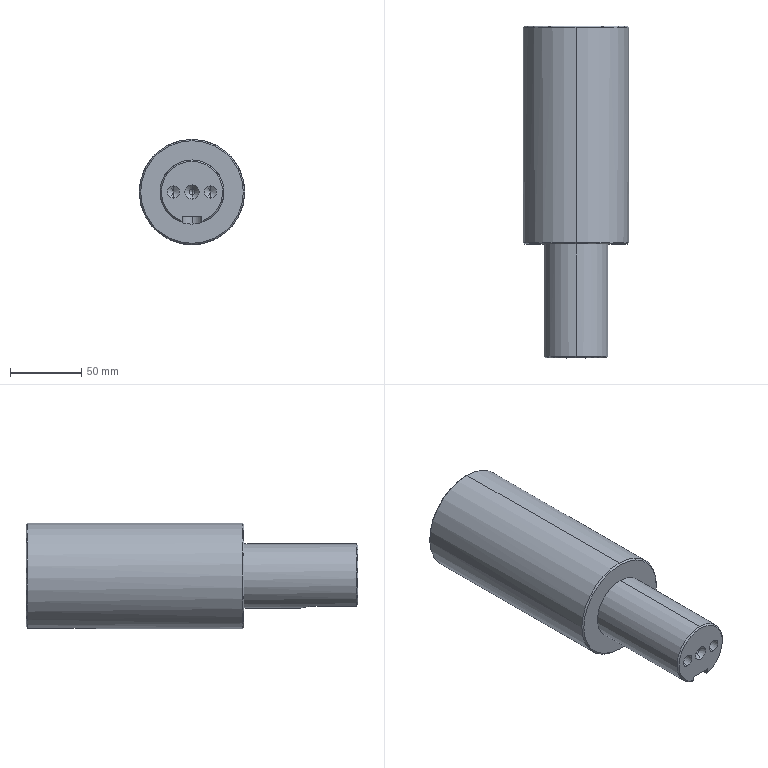Part | SolidWorks | features ICE 3, 3DProfileFeature 2, Chamfer 2, Fillet 2, HoleWzd 2, Extrusion 1 | 1 solid | 36 faces | box 74 x 233 x 74 mm | volume 776364 mm3 | cylinder 14 | cone 13 | plane 9 | commonest cylinder face diameters 8.5 x4 4 x2 10 x2 14 x2 45 x2 74 x2
STEP:
#1=CARTESIAN_POINT('',(0.,3.451,2.));
#2=VERTEX_POINT('',#1);
#3=CARTESIAN_POINT('',(0.,3.451,-2.));
#4=VERTEX_POINT('',#3);
#5=CARTESIAN_POINT('',(0.,3.451,0.));
#6=DIRECTION('',(0.,-1.,0.));
#7=DIRECTION('',(0.,0.,-1.));
#8=AXIS2_PLACEMENT_3D('',#5,#6,#7);
#9=CIRCLE('',#8,2.);
#10=EDGE_CURVE('',#2,#4,#9,.T.);
#11=ORIENTED_EDGE('',*,*,#10,.F.);
#12=CARTESIAN_POINT('',(0.,0.,5.));
#13=VERTEX_POINT('',#12);
#14=CARTESIAN_POINT('',(0.,0.,5.));
#15=DIRECTION('',(0.,-0.7547,0.6561));
#16=VECTOR('',#15,1000.);
#17=LINE('',#14,#16);
#18=EDGE_CURVE('',#2,#13,#17,.T.);
#19=ORIENTED_EDGE('',*,*,#18,.T.);
#20=CARTESIAN_POINT('',(0.,0.,-5.));
#21=VERTEX_POINT('',#20);
#22=CARTESIAN_POINT('',(0.,0.,0.));
#23=DIRECTION('',(0.,-1.,0.));
#24=DIRECTION('',(0.,0.,-1.));
#25=AXIS2_PLACEMENT_3D('',#22,#23,#24);
#26=CIRCLE('',#25,5.);
#27=EDGE_CURVE('',#13,#21,#26,.T.);
#28=ORIENTED_EDGE('',*,*,#27,.T.);
#29=CARTESIAN_POINT('',(0.,0.,-5.));
#30=DIRECTION('',(0.,-0.7547,-0.6561));
#31=VECTOR('',#30,1000.);
#32=LINE('',#29,#31);
#33=EDGE_CURVE('',#4,#21,#32,.T.);
#34=ORIENTED_EDGE('',*,*,#33,.F.);
#35=EDGE_LOOP('',(#11,#19,#28,#34));
#36=FACE_OUTER_BOUND('',#35,.T.);
#37=CARTESIAN_POINT('',(0.,0.,0.));
#38=DIRECTION('',(0.,-1.,0.));
#39=DIRECTION('',(0.,0.,-1.));
#40=AXIS2_PLACEMENT_3D('',#37,#38,#39);
#41=CONICAL_SURFACE('',#40,5.,0.7156);
#42=ADVANCED_FACE('',(#36),#41,.F.);
#43=CARTESIAN_POINT('',(0.,10.,2.));
#44=VERTEX_POINT('',#43);
#45=CARTESIAN_POINT('',(0.,10.,-2.));
#46=VERTEX_POINT('',#45);
#47=CARTESIAN_POINT('',(0.,10.,0.));
#48=DIRECTION('',(0.,-1.,0.));
#49=DIRECTION('',(0.,0.,-1.));
#50=AXIS2_PLACEMENT_3D('',#47,#48,#49);
#51=CIRCLE('',#50,2.);
#52=EDGE_CURVE('',#44,#46,#51,.T.);
#53=ORIENTED_EDGE('',*,*,#52,.F.);
#54=CARTESIAN_POINT('',(0.,0.,2.));
#55=DIRECTION('',(0.,-1.,0.));
#56=VECTOR('',#55,1000.);
#57=LINE('',#54,#56);
#58=EDGE_CURVE('',#44,#2,#57,.T.);
#59=ORIENTED_EDGE('',*,*,#58,.T.);
#60=ORIENTED_EDGE('',*,*,#10,.T.);
#61=CARTESIAN_POINT('',(0.,0.,-2.));
#62=DIRECTION('',(0.,-1.,0.));
#63=VECTOR('',#62,1000.);
#64=LINE('',#61,#63);
#65=EDGE_CURVE('',#46,#4,#64,.T.);
#66=ORIENTED_EDGE('',*,*,#65,.F.);
#67=EDGE_LOOP('',(#53,#59,#60,#66));
#68=FACE_OUTER_BOUND('',#67,.T.);
#69=CARTESIAN_POINT('',(0.,0.,0.));
#70=DIRECTION('',(0.,-1.,0.));
#71=DIRECTION('',(0.,0.,-1.));
#72=AXIS2_PLACEMENT_3D('',#69,#70,#71);
#73=CYLINDRICAL_SURFACE('',#72,2.);
#74=ADVANCED_FACE('',(#68),#73,.F.);
#75=CARTESIAN_POINT('',(0.,11.202,0.));
#76=VERTEX_POINT('',#75);
#77=CARTESIAN_POINT('',(0.,10.,-2.));
#78=DIRECTION('',(0.,-0.515,-0.8572));
#79=VECTOR('',#78,1000.);
#80=LINE('',#77,#79);
#81=EDGE_CURVE('',#76,#46,#80,.T.);
#82=ORIENTED_EDGE('',*,*,#81,.F.);
#83=CARTESIAN_POINT('',(0.,10.,2.));
#84=DIRECTION('',(0.,-0.515,0.8572));
#85=VECTOR('',#84,1000.);
#86=LINE('',#83,#85);
#87=EDGE_CURVE('',#76,#44,#86,.T.);
#88=ORIENTED_EDGE('',*,*,#87,.T.);
#89=ORIENTED_EDGE('',*,*,#52,.T.);
#90=EDGE_LOOP('',(#82,#88,#89));
#91=FACE_OUTER_BOUND('',#90,.T.);
#92=CARTESIAN_POINT('',(0.,10.,0.));
#93=DIRECTION('',(0.,-1.,0.));
#94=DIRECTION('',(0.,0.,-1.));
#95=AXIS2_PLACEMENT_3D('',#92,#93,#94);
#96=CONICAL_SURFACE('',#95,2.,1.03);
#97=ADVANCED_FACE('',(#91),#96,.F.);
#98=CARTESIAN_POINT('',(0.,80.,-36.));
#99=VERTEX_POINT('',#98);
#100=CARTESIAN_POINT('',(0.,80.,36.));
#101=VERTEX_POINT('',#100);
#102=CARTESIAN_POINT('',(0.,80.,0.));
#103=DIRECTION('',(0.,-1.,0.));
#104=DIRECTION('',(0.,0.,1.));
#105=AXIS2_PLACEMENT_3D('',#102,#103,#104);
#106=CIRCLE('',#105,36.);
#107=EDGE_CURVE('',#99,#101,#106,.T.);
#108=ORIENTED_EDGE('',*,*,#107,.F.);
#109=CARTESIAN_POINT('',(0.,81.,-37.));
#110=VERTEX_POINT('',#109);
#111=CARTESIAN_POINT('',(0.,81.,-37.));
#112=DIRECTION('',(0.,0.7071,-0.7071));
#113=VECTOR('',#112,1000.);
#114=LINE('',#111,#113);
#115=EDGE_CURVE('',#99,#110,#114,.T.);
#116=ORIENTED_EDGE('',*,*,#115,.T.);
#117=CARTESIAN_POINT('',(0.,81.,37.));
#118=VERTEX_POINT('',#117);
#119=CARTESIAN_POINT('',(0.,81.,0.));
#120=DIRECTION('',(0.,1.,0.));
#121=DIRECTION('',(0.,0.,1.));
#122=AXIS2_PLACEMENT_3D('',#119,#120,#121);
#123=CIRCLE('',#122,37.);
#124=EDGE_CURVE('',#118,#110,#123,.T.);
#125=ORIENTED_EDGE('',*,*,#124,.F.);
#126=CARTESIAN_POINT('',(0.,81.,37.));
#127=DIRECTION('',(0.,0.7071,0.7071));
#128=VECTOR('',#127,1000.);
#129=LINE('',#126,#128);
#130=EDGE_CURVE('',#101,#118,#129,.T.);
#131=ORIENTED_EDGE('',*,*,#130,.F.);
#132=EDGE_LOOP('',(#108,#116,#125,#131));
#133=FACE_OUTER_BOUND('',#132,.T.);
#134=CARTESIAN_POINT('',(0.,81.,0.));
#135=DIRECTION('',(0.,1.,0.));
#136=DIRECTION('',(0.,0.,1.));
#137=AXIS2_PLACEMENT_3D('',#134,#135,#136);
#138=CONICAL_SURFACE('',#137,37.,0.7854);
#139=ADVANCED_FACE('',(#133),#138,.T.);
#140=CARTESIAN_POINT('',(5.,232.,-36.661));
#141=VERTEX_POINT('',#140);
#142=CARTESIAN_POINT('',(0.,232.,37.));
#143=VERTEX_POINT('',#142);
#144=CARTESIAN_POINT('',(0.,232.,0.));
#145=DIRECTION('',(0.,-1.,0.));
#146=DIRECTION('',(0.,0.,1.));
#147=AXIS2_PLACEMENT_3D('',#144,#145,#146);
#148=CIRCLE('',#147,37.);
#149=EDGE_CURVE('',#141,#143,#148,.T.);
#150=ORIENTED_EDGE('',*,*,#149,.T.);
#151=CARTESIAN_POINT('',(0.,233.,37.));
#152=DIRECTION('',(0.,-1.,0.));
#153=VECTOR('',#152,1000.);
#154=LINE('',#151,#153);
#155=EDGE_CURVE('',#143,#118,#154,.T.);
#156=ORIENTED_EDGE('',*,*,#155,.T.);
#157=ORIENTED_EDGE('',*,*,#124,.T.);
#158=CARTESIAN_POINT('',(0.,183.,-37.));
#159=VERTEX_POINT('',#158);
#160=CARTESIAN_POINT('',(0.,233.,-37.));
#161=DIRECTION('',(0.,-1.,0.));
#162=VECTOR('',#161,1000.);
#163=LINE('',#160,#162);
#164=EDGE_CURVE('',#159,#110,#163,.T.);
#165=ORIENTED_EDGE('',*,*,#164,.F.);
#166=CARTESIAN_POINT('',(5.,188.,-36.661));
#167=VERTEX_POINT('',#166);
#168=CARTESIAN_POINT('',(0.,183.,-37.));
#169=CARTESIAN_POINT('',(0.3305,183.,-37.));
#170=CARTESIAN_POINT('',(0.6555,183.032,-36.996));
#171=CARTESIAN_POINT('',(1.135,183.128,-36.983));
#172=CARTESIAN_POINT('',(1.293,183.167,-36.978));
#173=CARTESIAN_POINT('',(1.607,183.263,-36.965));
#174=CARTESIAN_POINT('',(1.764,183.318,-36.958));
#175=CARTESIAN_POINT('',(2.217,183.507,-36.935));
#176=CARTESIAN_POINT('',(2.504,183.66,-36.916));
#177=CARTESIAN_POINT('',(3.047,184.022,-36.875));
#178=CARTESIAN_POINT('',(3.304,184.233,-36.853));
#179=CARTESIAN_POINT('',(3.765,184.693,-36.809));
#180=CARTESIAN_POINT('',(3.972,184.945,-36.787));
#181=CARTESIAN_POINT('',(4.337,185.491,-36.745));
#182=CARTESIAN_POINT('',(4.492,185.781,-36.726));
#183=CARTESIAN_POINT('',(4.742,186.382,-36.695));
#184=CARTESIAN_POINT('',(4.838,186.696,-36.682));
#185=CARTESIAN_POINT('',(4.968,187.343,-36.665));
#186=CARTESIAN_POINT('',(5.,187.669,-36.661));
#187=CARTESIAN_POINT('',(5.,188.,-36.661));
#188=B_SPLINE_CURVE_WITH_KNOTS('',3,(#168,#169,#170,#171,#172,#173,#174,#175,#176,#177,#178,#179,#180,#181,#182,#183,#184,#185,#186,#187),.UNSPECIFIED.,.F.,.F.,(4,2,2,2,2,2,2,2,2,4),(0.,0.0009775,0.001466,0.001955,0.002932,0.00391,0.004887,0.005865,0.006842,0.00782),.UNSPECIFIED.);
#189=EDGE_CURVE('',#159,#167,#188,.T.);
#190=ORIENTED_EDGE('',*,*,#189,.T.);
#191=CARTESIAN_POINT('',(5.,233.,-36.661));
#192=DIRECTION('',(0.,1.,0.));
#193=VECTOR('',#192,1000.);
#194=LINE('',#191,#193);
#195=EDGE_CURVE('',#167,#141,#194,.T.);
#196=ORIENTED_EDGE('',*,*,#195,.T.);
#197=EDGE_LOOP('',(#150,#156,#157,#165,#190,#196));
#198=FACE_OUTER_BOUND('',#197,.T.);
#199=CARTESIAN_POINT('',(0.,233.,0.));
#200=DIRECTION('',(0.,-1.,0.));
#201=DIRECTION('',(0.,0.,-1.));
#202=AXIS2_PLACEMENT_3D('',#199,#200,#201);
#203=CYLINDRICAL_SURFACE('',#202,37.);
#204=ADVANCED_FACE('',(#198),#203,.T.);
#205=CARTESIAN_POINT('',(0.,0.,21.5));
#206=VERTEX_POINT('',#205);
#207=CARTESIAN_POINT('',(-7.,0.,-20.329));
#208=VERTEX_POINT('',#207);
#209=CARTESIAN_POINT('',(0.,0.,0.));
#210=DIRECTION('',(0.,-1.,0.));
#211=DIRECTION('',(0.,0.,1.));
#212=AXIS2_PLACEMENT_3D('',#209,#210,#211);
#213=CIRCLE('',#212,21.5);
#214=EDGE_CURVE('',#206,#208,#213,.T.);
#215=ORIENTED_EDGE('',*,*,#214,.F.);
#216=CARTESIAN_POINT('',(0.,1.,22.5));
#217=VERTEX_POINT('',#216);
#218=CARTESIAN_POINT('',(0.,1.,22.5));
#219=DIRECTION('',(0.,0.7071,0.7071));
#220=VECTOR('',#219,1000.);
#221=LINE('',#218,#220);
#222=EDGE_CURVE('',#206,#217,#221,.T.);
#223=ORIENTED_EDGE('',*,*,#222,.T.);
#224=CARTESIAN_POINT('',(-7.,1.,-21.383));
#225=VERTEX_POINT('',#224);
#226=CARTESIAN_POINT('',(0.,1.,0.));
#227=DIRECTION('',(0.,1.,0.));
#228=DIRECTION('',(0.,0.,1.));
#229=AXIS2_PLACEMENT_3D('',#226,#227,#228);
#230=CIRCLE('',#229,22.5);
#231=EDGE_CURVE('',#225,#217,#230,.T.);
#232=ORIENTED_EDGE('',*,*,#231,.F.);
#233=CARTESIAN_POINT('',(-7.,0.,-20.329));
#234=CARTESIAN_POINT('',(-7.,0.3329,-20.681));
#235=CARTESIAN_POINT('',(-7.,0.6662,-21.032));
#236=CARTESIAN_POINT('',(-7.,1.,-21.383));
#237=B_SPLINE_CURVE_WITH_KNOTS('',3,(#233,#234,#235,#236),.UNSPECIFIED.,.F.,.F.,(4,4),(0.,0.001454),.UNSPECIFIED.);
#238=EDGE_CURVE('',#208,#225,#237,.T.);
#239=ORIENTED_EDGE('',*,*,#238,.F.);
#240=EDGE_LOOP('',(#215,#223,#232,#239));
#241=FACE_OUTER_BOUND('',#240,.T.);
#242=CARTESIAN_POINT('',(0.,1.,0.));
#243=DIRECTION('',(0.,1.,0.));
#244=DIRECTION('',(0.,0.,1.));
#245=AXIS2_PLACEMENT_3D('',#242,#243,#244);
#246=CONICAL_SURFACE('',#245,22.5,0.7854);
#247=ADVANCED_FACE('',(#241),#246,.T.);
#248=CARTESIAN_POINT('',(-13.,27.5,4.25));
#249=VERTEX_POINT('',#248);
#250=CARTESIAN_POINT('',(-13.,27.5,-4.25));
#251=VERTEX_POINT('',#250);
#252=CARTESIAN_POINT('',(-13.,27.5,0.));
#253=DIRECTION('',(0.,-1.,0.));
#254=DIRECTION('',(0.,0.,-1.));
#255=AXIS2_PLACEMENT_3D('',#252,#253,#254);
#256=CIRCLE('',#255,4.25);
#257=EDGE_CURVE('',#249,#251,#256,.T.);
#258=ORIENTED_EDGE('',*,*,#257,.F.);
#259=CARTESIAN_POINT('',(-13.,0.,4.25));
#260=VERTEX_POINT('',#259);
#261=CARTESIAN_POINT('',(-13.,0.,4.25));
#262=DIRECTION('',(0.,-1.,0.));
#263=VECTOR('',#262,1000.);
#264=LINE('',#261,#263);
#265=EDGE_CURVE('',#249,#260,#264,.T.);
#266=ORIENTED_EDGE('',*,*,#265,.T.);
#267=CARTESIAN_POINT('',(-13.,0.,-4.25));
#268=VERTEX_POINT('',#267);
#269=CARTESIAN_POINT('',(-13.,0.,0.));
#270=DIRECTION('',(0.,-1.,0.));
#271=DIRECTION('',(0.,0.,-1.));
#272=AXIS2_PLACEMENT_3D('',#269,#270,#271);
#273=CIRCLE('',#272,4.25);
#274=EDGE_CURVE('',#260,#268,#273,.T.);
#275=ORIENTED_EDGE('',*,*,#274,.T.);
#276=CARTESIAN_POINT('',(-13.,0.,-4.25));
#277=DIRECTION('',(0.,-1.,0.));
#278=VECTOR('',#277,1000.);
#279=LINE('',#276,#278);
#280=EDGE_CURVE('',#251,#268,#279,.T.);
#281=ORIENTED_EDGE('',*,*,#280,.F.);
#282=EDGE_LOOP('',(#258,#266,#275,#281));
#283=FACE_OUTER_BOUND('',#282,.T.);
#284=CARTESIAN_POINT('',(-13.,0.,0.));
#285=DIRECTION('',(0.,-1.,0.));
#286=DIRECTION('',(0.,0.,-1.));
#287=AXIS2_PLACEMENT_3D('',#284,#285,#286);
#288=CYLINDRICAL_SURFACE('',#287,4.25);
#289=ADVANCED_FACE('',(#283),#288,.F.);
#290=CARTESIAN_POINT('',(-13.,30.054,0.));
#291=VERTEX_POINT('',#290);
#292=CARTESIAN_POINT('',(-13.,27.5,-4.25));
#293=DIRECTION('',(0.,-0.515,-0.8572));
#294=VECTOR('',#293,1000.);
#295=LINE('',#292,#294);
#296=EDGE_CURVE('',#291,#251,#295,.T.);
#297=ORIENTED_EDGE('',*,*,#296,.F.);
#298=CARTESIAN_POINT('',(-13.,27.5,4.25));
#299=DIRECTION('',(0.,-0.515,0.8572));
#300=VECTOR('',#299,1000.);
#301=LINE('',#298,#300);
#302=EDGE_CURVE('',#291,#249,#301,.T.);
#303=ORIENTED_EDGE('',*,*,#302,.T.);
#304=ORIENTED_EDGE('',*,*,#257,.T.);
#305=EDGE_LOOP('',(#297,#303,#304));
#306=FACE_OUTER_BOUND('',#305,.T.);
#307=CARTESIAN_POINT('',(-13.,27.5,0.));
#308=DIRECTION('',(0.,-1.,0.));
#309=DIRECTION('',(0.,0.,-1.));
#310=AXIS2_PLACEMENT_3D('',#307,#308,#309);
#311=CONICAL_SURFACE('',#310,4.25,1.03);
#312=ADVANCED_FACE('',(#306),#311,.F.);
#313=CARTESIAN_POINT('',(13.,27.5,4.25));
#314=VERTEX_POINT('',#313);
#315=CARTESIAN_POINT('',(13.,27.5,-4.25));
#316=VERTEX_POINT('',#315);
#317=CARTESIAN_POINT('',(13.,27.5,0.));
#318=DIRECTION('',(0.,-1.,0.));
#319=DIRECTION('',(0.,0.,-1.));
#320=AXIS2_PLACEMENT_3D('',#317,#318,#319);
#321=CIRCLE('',#320,4.25);
#322=EDGE_CURVE('',#314,#316,#321,.T.);
#323=ORIENTED_EDGE('',*,*,#322,.F.);
#324=CARTESIAN_POINT('',(13.,0.,4.25));
#325=VERTEX_POINT('',#324);
#326=CARTESIAN_POINT('',(13.,0.,4.25));
#327=DIRECTION('',(0.,-1.,0.));
#328=VECTOR('',#327,1000.);
#329=LINE('',#326,#328);
#330=EDGE_CURVE('',#314,#325,#329,.T.);
#331=ORIENTED_EDGE('',*,*,#330,.T.);
#332=CARTESIAN_POINT('',(13.,0.,-4.25));
#333=VERTEX_POINT('',#332);
#334=CARTESIAN_POINT('',(13.,0.,0.));
#335=DIRECTION('',(0.,-1.,0.));
#336=DIRECTION('',(0.,0.,-1.));
#337=AXIS2_PLACEMENT_3D('',#334,#335,#336);
#338=CIRCLE('',#337,4.25);
#339=EDGE_CURVE('',#325,#333,#338,.T.);
#340=ORIENTED_EDGE('',*,*,#339,.T.);
#341=CARTESIAN_POINT('',(13.,0.,-4.25));
#342=DIRECTION('',(0.,-1.,0.));
#343=VECTOR('',#342,1000.);
#344=LINE('',#341,#343);
#345=EDGE_CURVE('',#316,#333,#344,.T.);
#346=ORIENTED_EDGE('',*,*,#345,.F.);
#347=EDGE_LOOP('',(#323,#331,#340,#346));
#348=FACE_OUTER_BOUND('',#347,.T.);
#349=CARTESIAN_POINT('',(13.,0.,0.));
#350=DIRECTION('',(0.,-1.,0.));
#351=DIRECTION('',(0.,0.,-1.));
#352=AXIS2_PLACEMENT_3D('',#349,#350,#351);
#353=CYLINDRICAL_SURFACE('',#352,4.25);
#354=ADVANCED_FACE('',(#348),#353,.F.);
#355=CARTESIAN_POINT('',(13.,30.054,0.));
#356=VERTEX_POINT('',#355);
#357=CARTESIAN_POINT('',(13.,27.5,-4.25));
#358=DIRECTION('',(0.,-0.515,-0.8572));
#359=VECTOR('',#358,1000.);
#360=LINE('',#357,#359);
#361=EDGE_CURVE('',#356,#316,#360,.T.);
#362=ORIENTED_EDGE('',*,*,#361,.F.);
#363=CARTESIAN_POINT('',(13.,27.5,4.25));
#364=DIRECTION('',(0.,-0.515,0.8572));
#365=VECTOR('',#364,1000.);
#366=LINE('',#363,#365);
#367=EDGE_CURVE('',#356,#314,#366,.T.);
#368=ORIENTED_EDGE('',*,*,#367,.T.);
#369=ORIENTED_EDGE('',*,*,#322,.T.);
#370=EDGE_LOOP('',(#362,#368,#369));
#371=FACE_OUTER_BOUND('',#370,.T.);
#372=CARTESIAN_POINT('',(13.,27.5,0.));
#373=DIRECTION('',(0.,-1.,0.));
#374=DIRECTION('',(0.,0.,-1.));
#375=AXIS2_PLACEMENT_3D('',#372,#373,#374);
#376=CONICAL_SURFACE('',#375,4.25,1.03);
#377=ADVANCED_FACE('',(#371),#376,.F.);
#378=CARTESIAN_POINT('',(0.,80.,22.5));
#379=VERTEX_POINT('',#378);
#380=CARTESIAN_POINT('',(0.,80.,-22.5));
#381=VERTEX_POINT('',#380);
#382=CARTESIAN_POINT('',(0.,80.,0.));
#383=DIRECTION('',(0.,1.,0.));
#384=DIRECTION('',(0.,0.,1.));
#385=AXIS2_PLACEMENT_3D('',#382,#383,#384);
#386=CIRCLE('',#385,22.5);
#387=EDGE_CURVE('',#379,#381,#386,.T.);
#388=ORIENTED_EDGE('',*,*,#387,.F.);
#389=CARTESIAN_POINT('',(0.,40.,22.5));
#390=DIRECTION('',(0.,-1.,0.));
#391=VECTOR('',#390,1000.);
#392=LINE('',#389,#391);
#393=EDGE_CURVE('',#379,#217,#392,.T.);
#394=ORIENTED_EDGE('',*,*,#393,.T.);
#395=CARTESIAN_POINT('',(7.,1.,-21.383));
#396=VERTEX_POINT('',#395);
#397=CARTESIAN_POINT('',(0.,1.,0.));
#398=DIRECTION('',(0.,1.,0.));
#399=DIRECTION('',(0.,0.,1.));
#400=AXIS2_PLACEMENT_3D('',#397,#398,#399);
#401=CIRCLE('',#400,22.5);
#402=EDGE_CURVE('',#217,#396,#401,.T.);
#403=ORIENTED_EDGE('',*,*,#402,.T.);
#404=CARTESIAN_POINT('',(7.,33.,-21.383));
#405=VERTEX_POINT('',#404);
#406=CARTESIAN_POINT('',(7.,40.,-21.383));
#407=DIRECTION('',(0.,-1.,0.));
#408=VECTOR('',#407,1000.);
#409=LINE('',#406,#408);
#410=EDGE_CURVE('',#405,#396,#409,.T.);
#411=ORIENTED_EDGE('',*,*,#410,.F.);
#412=CARTESIAN_POINT('',(0.,40.,-22.5));
#413=VERTEX_POINT('',#412);
#414=CARTESIAN_POINT('',(7.,33.,-21.383));
#415=CARTESIAN_POINT('',(7.,33.465,-21.383));
#416=CARTESIAN_POINT('',(6.954,33.922,-21.399));
#417=CARTESIAN_POINT('',(6.82,34.596,-21.442));
#418=CARTESIAN_POINT('',(6.764,34.818,-21.459));
#419=CARTESIAN_POINT('',(6.629,35.259,-21.501));
#420=CARTESIAN_POINT('',(6.551,35.478,-21.525));
#421=CARTESIAN_POINT('',(6.287,36.112,-21.605));
#422=CARTESIAN_POINT('',(6.072,36.513,-21.667));
#423=CARTESIAN_POINT('',(5.692,37.081,-21.769));
#424=CARTESIAN_POINT('',(5.554,37.266,-21.804));
#425=CARTESIAN_POINT('',(5.264,37.62,-21.876));
#426=CARTESIAN_POINT('',(5.112,37.788,-21.912));
#427=CARTESIAN_POINT('',(4.631,38.269,-22.021));
#428=CARTESIAN_POINT('',(4.281,38.558,-22.092));
#429=CARTESIAN_POINT('',(3.517,39.07,-22.227));
#430=CARTESIAN_POINT('',(3.115,39.285,-22.287));
#431=CARTESIAN_POINT('',(2.484,39.548,-22.363));
#432=CARTESIAN_POINT('',(2.269,39.626,-22.386));
#433=CARTESIAN_POINT('',(1.83,39.76,-22.427));
#434=CARTESIAN_POINT('',(1.604,39.818,-22.444));
#435=CARTESIAN_POINT('',(0.9245,39.954,-22.486));
#436=CARTESIAN_POINT('',(0.4653,40.,-22.5));
#437=CARTESIAN_POINT('',(0.,40.,-22.5));
#438=B_SPLINE_CURVE_WITH_KNOTS('',3,(#414,#415,#416,#417,#418,#419,#420,#421,#422,#423,#424,#425,#426,#427,#428,#429,#430,#431,#432,#433,#434,#435,#436,#437),.UNSPECIFIED.,.F.,.F.,(4,2,2,2,2,2,2,2,2,2,2,4),(0.,0.001375,0.002063,0.002751,0.004126,0.004814,0.005502,0.006877,0.008253,0.008941,0.009628,0.011),.UNSPECIFIED.);
#439=EDGE_CURVE('',#405,#413,#438,.T.);
#440=ORIENTED_EDGE('',*,*,#439,.T.);
#441=CARTESIAN_POINT('',(0.,40.,-22.5));
#442=DIRECTION('',(0.,-1.,0.));
#443=VECTOR('',#442,1000.);
#444=LINE('',#441,#443);
#445=EDGE_CURVE('',#381,#413,#444,.T.);
#446=ORIENTED_EDGE('',*,*,#445,.F.);
#447=EDGE_LOOP('',(#388,#394,#403,#411,#440,#446));
#448=FACE_OUTER_BOUND('',#447,.T.);
#449=CARTESIAN_POINT('',(0.,40.,0.));
#450=DIRECTION('',(0.,-1.,0.));
#451=DIRECTION('',(0.,0.,-1.));
#452=AXIS2_PLACEMENT_3D('',#449,#450,#451);
#453=CYLINDRICAL_SURFACE('',#452,22.5);
#454=ADVANCED_FACE('',(#448),#453,.T.);
#455=ORIENTED_EDGE('',*,*,#393,.F.);
#456=CARTESIAN_POINT('',(0.,80.,0.));
#457=DIRECTION('',(0.,1.,0.));
#458=DIRECTION('',(0.,0.,1.));
#459=AXIS2_PLACEMENT_3D('',#456,#457,#458);
#460=CIRCLE('',#459,22.5);
#461=EDGE_CURVE('',#381,#379,#460,.T.);
#462=ORIENTED_EDGE('',*,*,#461,.F.);
#463=ORIENTED_EDGE('',*,*,#445,.T.);
#464=CARTESIAN_POINT('',(-7.,33.,-21.383));
#465=VERTEX_POINT('',#464);
#466=CARTESIAN_POINT('',(0.,40.,-22.5));
#467=CARTESIAN_POINT('',(-0.4653,40.,-22.5));
#468=CARTESIAN_POINT('',(-0.9223,39.954,-22.486));
#469=CARTESIAN_POINT('',(-1.596,39.819,-22.444));
#470=CARTESIAN_POINT('',(-1.818,39.764,-22.427));
#471=CARTESIAN_POINT('',(-2.26,39.629,-22.387));
#472=CARTESIAN_POINT('',(-2.478,39.551,-22.364));
#473=CARTESIAN_POINT('',(-3.113,39.287,-22.288));
#474=CARTESIAN_POINT('',(-3.513,39.072,-22.227));
#475=CARTESIAN_POINT('',(-4.082,38.691,-22.127));
#476=CARTESIAN_POINT('',(-4.267,38.554,-22.092));
#477=CARTESIAN_POINT('',(-4.621,38.263,-22.021));
#478=CARTESIAN_POINT('',(-4.789,38.111,-21.985));
#479=CARTESIAN_POINT('',(-5.27,37.63,-21.877));
#480=CARTESIAN_POINT('',(-5.558,37.28,-21.804));
#481=CARTESIAN_POINT('',(-6.07,36.516,-21.667));
#482=CARTESIAN_POINT('',(-6.286,36.114,-21.605));
#483=CARTESIAN_POINT('',(-6.548,35.484,-21.526));
#484=CARTESIAN_POINT('',(-6.626,35.269,-21.502));
#485=CARTESIAN_POINT('',(-6.76,34.83,-21.46));
#486=CARTESIAN_POINT('',(-6.818,34.604,-21.442));
#487=CARTESIAN_POINT('',(-6.954,33.924,-21.399));
#488=CARTESIAN_POINT('',(-7.,33.465,-21.383));
#489=CARTESIAN_POINT('',(-7.,33.,-21.383));
#490=B_SPLINE_CURVE_WITH_KNOTS('',3,(#466,#467,#468,#469,#470,#471,#472,#473,#474,#475,#476,#477,#478,#479,#480,#481,#482,#483,#484,#485,#486,#487,#488,#489),.UNSPECIFIED.,.F.,.F.,(4,2,2,2,2,2,2,2,2,2,2,4),(0.,0.001376,0.002063,0.002751,0.004127,0.004814,0.005502,0.006878,0.008253,0.008941,0.009629,0.011),.UNSPECIFIED.);
#491=EDGE_CURVE('',#413,#465,#490,.T.);
#492=ORIENTED_EDGE('',*,*,#491,.T.);
#493=CARTESIAN_POINT('',(-7.,40.,-21.383));
#494=DIRECTION('',(0.,-1.,0.));
#495=VECTOR('',#494,1000.);
#496=LINE('',#493,#495);
#497=EDGE_CURVE('',#465,#225,#496,.T.);
#498=ORIENTED_EDGE('',*,*,#497,.T.);
#499=ORIENTED_EDGE('',*,*,#231,.T.);
#500=EDGE_LOOP('',(#455,#462,#463,#492,#498,#499));
#501=FACE_OUTER_BOUND('',#500,.T.);
#502=CARTESIAN_POINT('',(0.,40.,0.));
#503=DIRECTION('',(0.,-1.,0.));
#504=DIRECTION('',(0.,0.,-1.));
#505=AXIS2_PLACEMENT_3D('',#502,#503,#504);
#506=CYLINDRICAL_SURFACE('',#505,22.5);
#507=ADVANCED_FACE('',(#501),#506,.T.);
#508=ORIENTED_EDGE('',*,*,#410,.T.);
#509=CARTESIAN_POINT('',(7.,0.,-20.329));
#510=VERTEX_POINT('',#509);
#511=CARTESIAN_POINT('',(7.,1.,-21.383));
#512=CARTESIAN_POINT('',(7.,0.6662,-21.032));
#513=CARTESIAN_POINT('',(7.,0.3329,-20.681));
#514=CARTESIAN_POINT('',(7.,0.,-20.329));
#515=B_SPLINE_CURVE_WITH_KNOTS('',3,(#511,#512,#513,#514),.UNSPECIFIED.,.F.,.F.,(4,4),(0.,0.001454),.UNSPECIFIED.);
#516=EDGE_CURVE('',#396,#510,#515,.T.);
#517=ORIENTED_EDGE('',*,*,#516,.T.);
#518=CARTESIAN_POINT('',(7.,0.,-17.));
#519=VERTEX_POINT('',#518);
#520=CARTESIAN_POINT('',(7.,0.,-21.383));
#521=DIRECTION('',(0.,0.,1.));
#522=VECTOR('',#521,1000.);
#523=LINE('',#520,#522);
#524=EDGE_CURVE('',#510,#519,#523,.T.);
#525=ORIENTED_EDGE('',*,*,#524,.T.);
#526=CARTESIAN_POINT('',(7.,33.,-17.));
#527=VERTEX_POINT('',#526);
#528=CARTESIAN_POINT('',(7.,40.,-17.));
#529=DIRECTION('',(0.,-1.,0.));
#530=VECTOR('',#529,1000.);
#531=LINE('',#528,#530);
#532=EDGE_CURVE('',#527,#519,#531,.T.);
#533=ORIENTED_EDGE('',*,*,#532,.F.);
#534=CARTESIAN_POINT('',(7.,33.,-21.383));
#535=DIRECTION('',(0.,0.,-1.));
#536=VECTOR('',#535,1000.);
#537=LINE('',#534,#536);
#538=EDGE_CURVE('',#527,#405,#537,.T.);
#539=ORIENTED_EDGE('',*,*,#538,.T.);
#540=EDGE_LOOP('',(#508,#517,#525,#533,#539));
#541=FACE_OUTER_BOUND('',#540,.T.);
#542=CARTESIAN_POINT('',(7.,40.,-21.383));
#543=DIRECTION('',(1.,0.,0.));
#544=DIRECTION('',(0.,0.,-1.));
#545=AXIS2_PLACEMENT_3D('',#542,#543,#544);
#546=PLANE('',#545);
#547=ADVANCED_FACE('',(#541),#546,.F.);
#548=CARTESIAN_POINT('',(-7.,33.,-17.));
#549=VERTEX_POINT('',#548);
#550=CARTESIAN_POINT('',(-7.,0.,-17.));
#551=VERTEX_POINT('',#550);
#552=CARTESIAN_POINT('',(-7.,40.,-17.));
#553=DIRECTION('',(0.,-1.,0.));
#554=VECTOR('',#553,1000.);
#555=LINE('',#552,#554);
#556=EDGE_CURVE('',#549,#551,#555,.T.);
#557=ORIENTED_EDGE('',*,*,#556,.F.);
#558=CARTESIAN_POINT('',(0.,40.,-17.));
#559=VERTEX_POINT('',#558);
#560=CARTESIAN_POINT('',(0.,33.,-17.));
#561=DIRECTION('',(0.,0.,-1.));
#562=DIRECTION('',(1.,0.,0.));
#563=AXIS2_PLACEMENT_3D('',#560,#561,#562);
#564=CIRCLE('',#563,7.);
#565=EDGE_CURVE('',#549,#559,#564,.T.);
#566=ORIENTED_EDGE('',*,*,#565,.T.);
#567=CARTESIAN_POINT('',(0.,33.,-17.));
#568=DIRECTION('',(0.,0.,-1.));
#569=DIRECTION('',(1.,0.,0.));
#570=AXIS2_PLACEMENT_3D('',#567,#568,#569);
#571=CIRCLE('',#570,7.);
#572=EDGE_CURVE('',#559,#527,#571,.T.);
#573=ORIENTED_EDGE('',*,*,#572,.T.);
#574=ORIENTED_EDGE('',*,*,#532,.T.);
#575=CARTESIAN_POINT('',(-7.,0.,-17.));
#576=DIRECTION('',(-1.,0.,0.));
#577=VECTOR('',#576,1000.);
#578=LINE('',#575,#577);
#579=EDGE_CURVE('',#519,#551,#578,.T.);
#580=ORIENTED_EDGE('',*,*,#579,.T.);
#581=EDGE_LOOP('',(#557,#566,#573,#574,#580));
#582=FACE_OUTER_BOUND('',#581,.T.);
#583=CARTESIAN_POINT('',(-7.,40.,-17.));
#584=DIRECTION('',(0.,0.,1.));
#585=DIRECTION('',(1.,0.,0.));
#586=AXIS2_PLACEMENT_3D('',#583,#584,#585);
#587=PLANE('',#586);
#588=ADVANCED_FACE('',(#582),#587,.F.);
#589=CARTESIAN_POINT('',(-7.,0.,-21.383));
#590=DIRECTION('',(0.,0.,-1.));
#591=VECTOR('',#590,1000.);
#592=LINE('',#589,#591);
#593=EDGE_CURVE('',#551,#208,#592,.T.);
#594=ORIENTED_EDGE('',*,*,#593,.T.);
#595=ORIENTED_EDGE('',*,*,#238,.T.);
#596=ORIENTED_EDGE('',*,*,#497,.F.);
#597=CARTESIAN_POINT('',(-7.,33.,-17.));
#598=DIRECTION('',(0.,0.,1.));
#599=VECTOR('',#598,1000.);
#600=LINE('',#597,#599);
#601=EDGE_CURVE('',#465,#549,#600,.T.);
#602=ORIENTED_EDGE('',*,*,#601,.T.);
#603=ORIENTED_EDGE('',*,*,#556,.T.);
#604=EDGE_LOOP('',(#594,#595,#596,#602,#603));
#605=FACE_OUTER_BOUND('',#604,.T.);
#606=CARTESIAN_POINT('',(-7.,40.,-21.383));
#607=DIRECTION('',(-1.,0.,0.));
#608=DIRECTION('',(0.,0.,1.));
#609=AXIS2_PLACEMENT_3D('',#606,#607,#608);
#610=PLANE('',#609);
#611=ADVANCED_FACE('',(#605),#610,.F.);
#612=CARTESIAN_POINT('',(0.,0.,0.));
#613=DIRECTION('',(0.,-1.,0.));
#614=DIRECTION('',(0.,0.,-1.));
#615=AXIS2_PLACEMENT_3D('',#612,#613,#614);
#616=CIRCLE('',#615,5.);
#617=EDGE_CURVE('',#21,#13,#616,.T.);
#618=ORIENTED_EDGE('',*,*,#617,.F.);
#619=ORIENTED_EDGE('',*,*,#27,.F.);
#620=EDGE_LOOP('',(#618,#619));
#621=FACE_BOUND('',#620,.T.);
#622=CARTESIAN_POINT('',(-13.,0.,0.));
#623=DIRECTION('',(0.,-1.,0.));
#624=DIRECTION('',(0.,0.,-1.));
#625=AXIS2_PLACEMENT_3D('',#622,#623,#624);
#626=CIRCLE('',#625,4.25);
#627=EDGE_CURVE('',#268,#260,#626,.T.);
#628=ORIENTED_EDGE('',*,*,#627,.F.);
#629=ORIENTED_EDGE('',*,*,#274,.F.);
#630=EDGE_LOOP('',(#628,#629));
#631=FACE_BOUND('',#630,.T.);
#632=CARTESIAN_POINT('',(13.,0.,0.));
#633=DIRECTION('',(0.,-1.,0.));
#634=DIRECTION('',(0.,0.,-1.));
#635=AXIS2_PLACEMENT_3D('',#632,#633,#634);
#636=CIRCLE('',#635,4.25);
#637=EDGE_CURVE('',#333,#325,#636,.T.);
#638=ORIENTED_EDGE('',*,*,#637,.F.);
#639=ORIENTED_EDGE('',*,*,#339,.F.);
#640=EDGE_LOOP('',(#638,#639));
#641=FACE_BOUND('',#640,.T.);
#642=ORIENTED_EDGE('',*,*,#524,.F.);
#643=CARTESIAN_POINT('',(0.,0.,0.));
#644=DIRECTION('',(0.,-1.,0.));
#645=DIRECTION('',(0.,0.,1.));
#646=AXIS2_PLACEMENT_3D('',#643,#644,#645);
#647=CIRCLE('',#646,21.5);
#648=EDGE_CURVE('',#510,#206,#647,.T.);
#649=ORIENTED_EDGE('',*,*,#648,.T.);
#650=ORIENTED_EDGE('',*,*,#214,.T.);
#651=ORIENTED_EDGE('',*,*,#593,.F.);
#652=ORIENTED_EDGE('',*,*,#579,.F.);
#653=EDGE_LOOP('',(#642,#649,#650,#651,#652));
#654=FACE_OUTER_BOUND('',#653,.T.);
#655=CARTESIAN_POINT('',(0.,0.,0.));
#656=DIRECTION('',(0.,1.,0.));
#657=DIRECTION('',(0.,0.,1.));
#658=AXIS2_PLACEMENT_3D('',#655,#656,#657);
#659=PLANE('',#658);
#660=ADVANCED_FACE('',(#621,#631,#641,#654),#659,.F.);
#661=ORIENTED_EDGE('',*,*,#367,.F.);
#662=ORIENTED_EDGE('',*,*,#361,.T.);
#663=CARTESIAN_POINT('',(13.,27.5,0.));
#664=DIRECTION('',(0.,-1.,0.));
#665=DIRECTION('',(0.,0.,-1.));
#666=AXIS2_PLACEMENT_3D('',#663,#664,#665);
#667=CIRCLE('',#666,4.25);
#668=EDGE_CURVE('',#316,#314,#667,.T.);
#669=ORIENTED_EDGE('',*,*,#668,.T.);
#670=EDGE_LOOP('',(#661,#662,#669));
#671=FACE_OUTER_BOUND('',#670,.T.);
#672=CARTESIAN_POINT('',(13.,27.5,0.));
#673=DIRECTION('',(0.,-1.,0.));
#674=DIRECTION('',(0.,0.,-1.));
#675=AXIS2_PLACEMENT_3D('',#672,#673,#674);
#676=CONICAL_SURFACE('',#675,4.25,1.03);
#677=ADVANCED_FACE('',(#671),#676,.F.);
#678=ORIENTED_EDGE('',*,*,#330,.F.);
#679=ORIENTED_EDGE('',*,*,#668,.F.);
#680=ORIENTED_EDGE('',*,*,#345,.T.);
#681=ORIENTED_EDGE('',*,*,#637,.T.);
#682=EDGE_LOOP('',(#678,#679,#680,#681));
#683=FACE_OUTER_BOUND('',#682,.T.);
#684=CARTESIAN_POINT('',(13.,0.,0.));
#685=DIRECTION('',(0.,-1.,0.));
#686=DIRECTION('',(0.,0.,-1.));
#687=AXIS2_PLACEMENT_3D('',#684,#685,#686);
#688=CYLINDRICAL_SURFACE('',#687,4.25);
#689=ADVANCED_FACE('',(#683),#688,.F.);
#690=ORIENTED_EDGE('',*,*,#302,.F.);
#691=ORIENTED_EDGE('',*,*,#296,.T.);
#692=CARTESIAN_POINT('',(-13.,27.5,0.));
#693=DIRECTION('',(0.,-1.,0.));
#694=DIRECTION('',(0.,0.,-1.));
#695=AXIS2_PLACEMENT_3D('',#692,#693,#694);
#696=CIRCLE('',#695,4.25);
#697=EDGE_CURVE('',#251,#249,#696,.T.);
#698=ORIENTED_EDGE('',*,*,#697,.T.);
#699=EDGE_LOOP('',(#690,#691,#698));
#700=FACE_OUTER_BOUND('',#699,.T.);
#701=CARTESIAN_POINT('',(-13.,27.5,0.));
#702=DIRECTION('',(0.,-1.,0.));
#703=DIRECTION('',(0.,0.,-1.));
#704=AXIS2_PLACEMENT_3D('',#701,#702,#703);
#705=CONICAL_SURFACE('',#704,4.25,1.03);
#706=ADVANCED_FACE('',(#700),#705,.F.);
#707=ORIENTED_EDGE('',*,*,#265,.F.);
#708=ORIENTED_EDGE('',*,*,#697,.F.);
#709=ORIENTED_EDGE('',*,*,#280,.T.);
#710=ORIENTED_EDGE('',*,*,#627,.T.);
#711=EDGE_LOOP('',(#707,#708,#709,#710));
#712=FACE_OUTER_BOUND('',#711,.T.);
#713=CARTESIAN_POINT('',(-13.,0.,0.));
#714=DIRECTION('',(0.,-1.,0.));
#715=DIRECTION('',(0.,0.,-1.));
#716=AXIS2_PLACEMENT_3D('',#713,#714,#715);
#717=CYLINDRICAL_SURFACE('',#716,4.25);
#718=ADVANCED_FACE('',(#712),#717,.F.);
#719=ORIENTED_EDGE('',*,*,#538,.F.);
#720=ORIENTED_EDGE('',*,*,#572,.F.);
#721=CARTESIAN_POINT('',(0.,40.,-17.));
#722=DIRECTION('',(0.,0.,1.));
#723=VECTOR('',#722,1000.);
#724=LINE('',#721,#723);
#725=EDGE_CURVE('',#413,#559,#724,.T.);
#726=ORIENTED_EDGE('',*,*,#725,.F.);
#727=ORIENTED_EDGE('',*,*,#439,.F.);
#728=EDGE_LOOP('',(#719,#720,#726,#727));
#729=FACE_OUTER_BOUND('',#728,.T.);
#730=CARTESIAN_POINT('',(0.,33.,0.));
#731=DIRECTION('',(0.,0.,-1.));
#732=DIRECTION('',(-1.,0.,0.));
#733=AXIS2_PLACEMENT_3D('',#730,#731,#732);
#734=CYLINDRICAL_SURFACE('',#733,7.);
#735=ADVANCED_FACE('',(#729),#734,.F.);
#736=ORIENTED_EDGE('',*,*,#565,.F.);
#737=ORIENTED_EDGE('',*,*,#601,.F.);
#738=ORIENTED_EDGE('',*,*,#491,.F.);
#739=ORIENTED_EDGE('',*,*,#725,.T.);
#740=EDGE_LOOP('',(#736,#737,#738,#739));
#741=FACE_OUTER_BOUND('',#740,.T.);
#742=CARTESIAN_POINT('',(0.,33.,0.));
#743=DIRECTION('',(0.,0.,1.));
#744=DIRECTION('',(1.,0.,0.));
#745=AXIS2_PLACEMENT_3D('',#742,#743,#744);
#746=CYLINDRICAL_SURFACE('',#745,7.);
#747=ADVANCED_FACE('',(#741),#746,.F.);
#748=ORIENTED_EDGE('',*,*,#222,.F.);
#749=ORIENTED_EDGE('',*,*,#648,.F.);
#750=ORIENTED_EDGE('',*,*,#516,.F.);
#751=ORIENTED_EDGE('',*,*,#402,.F.);
#752=EDGE_LOOP('',(#748,#749,#750,#751));
#753=FACE_OUTER_BOUND('',#752,.T.);
#754=CARTESIAN_POINT('',(0.,1.,0.));
#755=DIRECTION('',(0.,1.,0.));
#756=DIRECTION('',(0.,0.,1.));
#757=AXIS2_PLACEMENT_3D('',#754,#755,#756);
#758=CONICAL_SURFACE('',#757,22.5,0.7854);
#759=ADVANCED_FACE('',(#753),#758,.T.);
#760=ORIENTED_EDGE('',*,*,#155,.F.);
#761=CARTESIAN_POINT('',(-5.,232.,-36.661));
#762=VERTEX_POINT('',#761);
#763=CARTESIAN_POINT('',(0.,232.,0.));
#764=DIRECTION('',(0.,-1.,0.));
#765=DIRECTION('',(0.,0.,1.));
#766=AXIS2_PLACEMENT_3D('',#763,#764,#765);
#767=CIRCLE('',#766,37.);
#768=EDGE_CURVE('',#143,#762,#767,.T.);
#769=ORIENTED_EDGE('',*,*,#768,.T.);
#770=CARTESIAN_POINT('',(-5.,188.,-36.661));
#771=VERTEX_POINT('',#770);
#772=CARTESIAN_POINT('',(-5.,233.,-36.661));
#773=DIRECTION('',(0.,-1.,0.));
#774=VECTOR('',#773,1000.);
#775=LINE('',#772,#774);
#776=EDGE_CURVE('',#762,#771,#775,.T.);
#777=ORIENTED_EDGE('',*,*,#776,.T.);
#778=CARTESIAN_POINT('',(-5.,188.,-36.661));
#779=CARTESIAN_POINT('',(-5.,187.669,-36.661));
#780=CARTESIAN_POINT('',(-4.968,187.345,-36.665));
#781=CARTESIAN_POINT('',(-4.872,186.865,-36.678));
#782=CARTESIAN_POINT('',(-4.833,186.707,-36.683));
#783=CARTESIAN_POINT('',(-4.737,186.393,-36.695));
#784=CARTESIAN_POINT('',(-4.682,186.236,-36.703));
#785=CARTESIAN_POINT('',(-4.493,185.783,-36.726));
#786=CARTESIAN_POINT('',(-4.34,185.496,-36.745));
#787=CARTESIAN_POINT('',(-3.978,184.953,-36.786));
#788=CARTESIAN_POINT('',(-3.767,184.696,-36.808));
#789=CARTESIAN_POINT('',(-3.307,184.235,-36.853));
#790=CARTESIAN_POINT('',(-3.055,184.029,-36.875));
#791=CARTESIAN_POINT('',(-2.51,183.663,-36.916));
#792=CARTESIAN_POINT('',(-2.219,183.508,-36.935));
#793=CARTESIAN_POINT('',(-1.618,183.258,-36.966));
#794=CARTESIAN_POINT('',(-1.304,183.162,-36.978));
#795=CARTESIAN_POINT('',(-0.6573,183.032,-36.996));
#796=CARTESIAN_POINT('',(-0.3305,183.,-37.));
#797=CARTESIAN_POINT('',(0.,183.,-37.));
#798=B_SPLINE_CURVE_WITH_KNOTS('',3,(#778,#779,#780,#781,#782,#783,#784,#785,#786,#787,#788,#789,#790,#791,#792,#793,#794,#795,#796,#797),.UNSPECIFIED.,.F.,.F.,(4,2,2,2,2,2,2,2,2,4),(0.,0.0009775,0.001466,0.001955,0.002932,0.00391,0.004887,0.005865,0.006842,0.00782),.UNSPECIFIED.);
#799=EDGE_CURVE('',#771,#159,#798,.T.);
#800=ORIENTED_EDGE('',*,*,#799,.T.);
#801=ORIENTED_EDGE('',*,*,#164,.T.);
#802=CARTESIAN_POINT('',(0.,81.,0.));
#803=DIRECTION('',(0.,1.,0.));
#804=DIRECTION('',(0.,0.,1.));
#805=AXIS2_PLACEMENT_3D('',#802,#803,#804);
#806=CIRCLE('',#805,37.);
#807=EDGE_CURVE('',#110,#118,#806,.T.);
#808=ORIENTED_EDGE('',*,*,#807,.T.);
#809=EDGE_LOOP('',(#760,#769,#777,#800,#801,#808));
#810=FACE_OUTER_BOUND('',#809,.T.);
#811=CARTESIAN_POINT('',(0.,233.,0.));
#812=DIRECTION('',(0.,-1.,0.));
#813=DIRECTION('',(0.,0.,-1.));
#814=AXIS2_PLACEMENT_3D('',#811,#812,#813);
#815=CYLINDRICAL_SURFACE('',#814,37.);
#816=ADVANCED_FACE('',(#810),#815,.T.);
#817=CARTESIAN_POINT('',(5.,233.,-32.));
#818=VERTEX_POINT('',#817);
#819=CARTESIAN_POINT('',(5.,233.,-35.651));
#820=VERTEX_POINT('',#819);
#821=CARTESIAN_POINT('',(5.,233.,-40.));
#822=DIRECTION('',(0.,0.,-1.));
#823=VECTOR('',#822,1000.);
#824=LINE('',#821,#823);
#825=EDGE_CURVE('',#818,#820,#824,.T.);
#826=ORIENTED_EDGE('',*,*,#825,.F.);
#827=CARTESIAN_POINT('',(-5.,233.,-32.));
#828=VERTEX_POINT('',#827);
#829=CARTESIAN_POINT('',(5.,233.,-32.));
#830=DIRECTION('',(1.,0.,0.));
#831=VECTOR('',#830,1000.);
#832=LINE('',#829,#831);
#833=EDGE_CURVE('',#828,#818,#832,.T.);
#834=ORIENTED_EDGE('',*,*,#833,.F.);
#835=CARTESIAN_POINT('',(-5.,233.,-35.651));
#836=VERTEX_POINT('',#835);
#837=CARTESIAN_POINT('',(-5.,233.,-40.));
#838=DIRECTION('',(0.,0.,1.));
#839=VECTOR('',#838,1000.);
#840=LINE('',#837,#839);
#841=EDGE_CURVE('',#836,#828,#840,.T.);
#842=ORIENTED_EDGE('',*,*,#841,.F.);
#843=CARTESIAN_POINT('',(0.,233.,0.));
#844=DIRECTION('',(0.,1.,0.));
#845=DIRECTION('',(0.,0.,1.));
#846=AXIS2_PLACEMENT_3D('',#843,#844,#845);
#847=CIRCLE('',#846,36.);
#848=EDGE_CURVE('',#836,#820,#847,.T.);
#849=ORIENTED_EDGE('',*,*,#848,.T.);
#850=EDGE_LOOP('',(#826,#834,#842,#849));
#851=FACE_OUTER_BOUND('',#850,.T.);
#852=CARTESIAN_POINT('',(0.,233.,0.));
#853=DIRECTION('',(0.,1.,0.));
#854=DIRECTION('',(0.,0.,1.));
#855=AXIS2_PLACEMENT_3D('',#852,#853,#854);
#856=PLANE('',#855);
#857=ADVANCED_FACE('',(#851),#856,.T.);
#858=CARTESIAN_POINT('',(0.,80.,0.));
#859=DIRECTION('',(0.,-1.,0.));
#860=DIRECTION('',(0.,0.,1.));
#861=AXIS2_PLACEMENT_3D('',#858,#859,#860);
#862=CIRCLE('',#861,36.);
#863=EDGE_CURVE('',#101,#99,#862,.T.);
#864=ORIENTED_EDGE('',*,*,#863,.T.);
#865=ORIENTED_EDGE('',*,*,#107,.T.);
#866=EDGE_LOOP('',(#864,#865));
#867=FACE_OUTER_BOUND('',#866,.T.);
#868=ORIENTED_EDGE('',*,*,#461,.T.);
#869=ORIENTED_EDGE('',*,*,#387,.T.);
#870=EDGE_LOOP('',(#868,#869));
#871=FACE_BOUND('',#870,.T.);
#872=CARTESIAN_POINT('',(0.,80.,0.));
#873=DIRECTION('',(0.,1.,0.));
#874=DIRECTION('',(0.,0.,1.));
#875=AXIS2_PLACEMENT_3D('',#872,#873,#874);
#876=PLANE('',#875);
#877=ADVANCED_FACE('',(#867,#871),#876,.F.);
#878=CARTESIAN_POINT('',(5.,233.,-35.651));
#879=CARTESIAN_POINT('',(5.,232.667,-35.988));
#880=CARTESIAN_POINT('',(5.,232.333,-36.324));
#881=CARTESIAN_POINT('',(5.,232.,-36.661));
#882=B_SPLINE_CURVE_WITH_KNOTS('',3,(#878,#879,#880,#881),.UNSPECIFIED.,.F.,.F.,(4,4),(0.007253,0.008674),.UNSPECIFIED.);
#883=EDGE_CURVE('',#820,#141,#882,.T.);
#884=ORIENTED_EDGE('',*,*,#883,.F.);
#885=ORIENTED_EDGE('',*,*,#848,.F.);
#886=CARTESIAN_POINT('',(-5.,232.,-36.661));
#887=CARTESIAN_POINT('',(-5.,232.333,-36.324));
#888=CARTESIAN_POINT('',(-5.,232.667,-35.988));
#889=CARTESIAN_POINT('',(-5.,233.,-35.651));
#890=B_SPLINE_CURVE_WITH_KNOTS('',3,(#886,#887,#888,#889),.UNSPECIFIED.,.F.,.F.,(4,4),(0.007241,0.008662),.UNSPECIFIED.);
#891=EDGE_CURVE('',#762,#836,#890,.T.);
#892=ORIENTED_EDGE('',*,*,#891,.F.);
#893=ORIENTED_EDGE('',*,*,#768,.F.);
#894=ORIENTED_EDGE('',*,*,#149,.F.);
#895=EDGE_LOOP('',(#884,#885,#892,#893,#894));
#896=FACE_OUTER_BOUND('',#895,.T.);
#897=CARTESIAN_POINT('',(0.,233.,0.));
#898=DIRECTION('',(0.,-1.,0.));
#899=DIRECTION('',(0.,0.,-1.));
#900=AXIS2_PLACEMENT_3D('',#897,#898,#899);
#901=CONICAL_SURFACE('',#900,36.,0.7854);
#902=ADVANCED_FACE('',(#896),#901,.T.);
#903=ORIENTED_EDGE('',*,*,#115,.F.);
#904=ORIENTED_EDGE('',*,*,#863,.F.);
#905=ORIENTED_EDGE('',*,*,#130,.T.);
#906=ORIENTED_EDGE('',*,*,#807,.F.);
#907=EDGE_LOOP('',(#903,#904,#905,#906));
#908=FACE_OUTER_BOUND('',#907,.T.);
#909=CARTESIAN_POINT('',(0.,81.,0.));
#910=DIRECTION('',(0.,1.,0.));
#911=DIRECTION('',(0.,0.,1.));
#912=AXIS2_PLACEMENT_3D('',#909,#910,#911);
#913=CONICAL_SURFACE('',#912,37.,0.7854);
#914=ADVANCED_FACE('',(#908),#913,.T.);
#915=ORIENTED_EDGE('',*,*,#87,.F.);
#916=ORIENTED_EDGE('',*,*,#81,.T.);
#917=CARTESIAN_POINT('',(0.,10.,0.));
#918=DIRECTION('',(0.,-1.,0.));
#919=DIRECTION('',(0.,0.,-1.));
#920=AXIS2_PLACEMENT_3D('',#917,#918,#919);
#921=CIRCLE('',#920,2.);
#922=EDGE_CURVE('',#46,#44,#921,.T.);
#923=ORIENTED_EDGE('',*,*,#922,.T.);
#924=EDGE_LOOP('',(#915,#916,#923));
#925=FACE_OUTER_BOUND('',#924,.T.);
#926=CARTESIAN_POINT('',(0.,10.,0.));
#927=DIRECTION('',(0.,-1.,0.));
#928=DIRECTION('',(0.,0.,-1.));
#929=AXIS2_PLACEMENT_3D('',#926,#927,#928);
#930=CONICAL_SURFACE('',#929,2.,1.03);
#931=ADVANCED_FACE('',(#925),#930,.F.);
#932=ORIENTED_EDGE('',*,*,#58,.F.);
#933=ORIENTED_EDGE('',*,*,#922,.F.);
#934=ORIENTED_EDGE('',*,*,#65,.T.);
#935=CARTESIAN_POINT('',(0.,3.451,0.));
#936=DIRECTION('',(0.,-1.,0.));
#937=DIRECTION('',(0.,0.,-1.));
#938=AXIS2_PLACEMENT_3D('',#935,#936,#937);
#939=CIRCLE('',#938,2.);
#940=EDGE_CURVE('',#4,#2,#939,.T.);
#941=ORIENTED_EDGE('',*,*,#940,.T.);
#942=EDGE_LOOP('',(#932,#933,#934,#941));
#943=FACE_OUTER_BOUND('',#942,.T.);
#944=CARTESIAN_POINT('',(0.,0.,0.));
#945=DIRECTION('',(0.,-1.,0.));
#946=DIRECTION('',(0.,0.,-1.));
#947=AXIS2_PLACEMENT_3D('',#944,#945,#946);
#948=CYLINDRICAL_SURFACE('',#947,2.);
#949=ADVANCED_FACE('',(#943),#948,.F.);
#950=ORIENTED_EDGE('',*,*,#18,.F.);
#951=ORIENTED_EDGE('',*,*,#940,.F.);
#952=ORIENTED_EDGE('',*,*,#33,.T.);
#953=ORIENTED_EDGE('',*,*,#617,.T.);
#954=EDGE_LOOP('',(#950,#951,#952,#953));
#955=FACE_OUTER_BOUND('',#954,.T.);
#956=CARTESIAN_POINT('',(0.,0.,0.));
#957=DIRECTION('',(0.,-1.,0.));
#958=DIRECTION('',(0.,0.,-1.));
#959=AXIS2_PLACEMENT_3D('',#956,#957,#958);
#960=CONICAL_SURFACE('',#959,5.,0.7156);
#961=ADVANCED_FACE('',(#955),#960,.F.);
#962=ORIENTED_EDGE('',*,*,#195,.F.);
#963=CARTESIAN_POINT('',(5.,188.,-32.));
#964=VERTEX_POINT('',#963);
#965=CARTESIAN_POINT('',(5.,188.,-32.));
#966=DIRECTION('',(0.,0.,1.));
#967=VECTOR('',#966,1000.);
#968=LINE('',#965,#967);
#969=EDGE_CURVE('',#167,#964,#968,.T.);
#970=ORIENTED_EDGE('',*,*,#969,.T.);
#971=CARTESIAN_POINT('',(5.,183.,-32.));
#972=DIRECTION('',(0.,1.,0.));
#973=VECTOR('',#972,1000.);
#974=LINE('',#971,#973);
#975=EDGE_CURVE('',#964,#818,#974,.T.);
#976=ORIENTED_EDGE('',*,*,#975,.T.);
#977=ORIENTED_EDGE('',*,*,#825,.T.);
#978=ORIENTED_EDGE('',*,*,#883,.T.);
#979=EDGE_LOOP('',(#962,#970,#976,#977,#978));
#980=FACE_OUTER_BOUND('',#979,.T.);
#981=CARTESIAN_POINT('',(5.,183.,-40.));
#982=DIRECTION('',(1.,0.,0.));
#983=DIRECTION('',(0.,0.,-1.));
#984=AXIS2_PLACEMENT_3D('',#981,#982,#983);
#985=PLANE('',#984);
#986=ADVANCED_FACE('',(#980),#985,.F.);
#987=CARTESIAN_POINT('',(-5.,188.,-32.));
#988=VERTEX_POINT('',#987);
#989=CARTESIAN_POINT('',(-5.,183.,-32.));
#990=DIRECTION('',(0.,1.,0.));
#991=VECTOR('',#990,1000.);
#992=LINE('',#989,#991);
#993=EDGE_CURVE('',#988,#828,#992,.T.);
#994=ORIENTED_EDGE('',*,*,#993,.F.);
#995=CARTESIAN_POINT('',(-5.,188.,-36.661));
#996=DIRECTION('',(0.,0.,-1.));
#997=VECTOR('',#996,1000.);
#998=LINE('',#995,#997);
#999=EDGE_CURVE('',#988,#771,#998,.T.);
#1000=ORIENTED_EDGE('',*,*,#999,.T.);
#1001=ORIENTED_EDGE('',*,*,#776,.F.);
#1002=ORIENTED_EDGE('',*,*,#891,.T.);
#1003=ORIENTED_EDGE('',*,*,#841,.T.);
#1004=EDGE_LOOP('',(#994,#1000,#1001,#1002,#1003));
#1005=FACE_OUTER_BOUND('',#1004,.T.);
#1006=CARTESIAN_POINT('',(-5.,183.,-40.));
#1007=DIRECTION('',(-1.,0.,0.));
#1008=DIRECTION('',(0.,0.,1.));
#1009=AXIS2_PLACEMENT_3D('',#1006,#1007,#1008);
#1010=PLANE('',#1009);
#1011=ADVANCED_FACE('',(#1005),#1010,.F.);
#1012=CARTESIAN_POINT('',(0.,183.,-32.));
#1013=VERTEX_POINT('',#1012);
#1014=CARTESIAN_POINT('',(0.,188.,-32.));
#1015=DIRECTION('',(0.,0.,-1.));
#1016=DIRECTION('',(1.,0.,0.));
#1017=AXIS2_PLACEMENT_3D('',#1014,#1015,#1016);
#1018=CIRCLE('',#1017,5.);
#1019=EDGE_CURVE('',#964,#1013,#1018,.T.);
#1020=ORIENTED_EDGE('',*,*,#1019,.T.);
#1021=CARTESIAN_POINT('',(0.,188.,-32.));
#1022=DIRECTION('',(0.,0.,-1.));
#1023=DIRECTION('',(1.,0.,0.));
#1024=AXIS2_PLACEMENT_3D('',#1021,#1022,#1023);
#1025=CIRCLE('',#1024,5.);
#1026=EDGE_CURVE('',#1013,#988,#1025,.T.);
#1027=ORIENTED_EDGE('',*,*,#1026,.T.);
#1028=ORIENTED_EDGE('',*,*,#993,.T.);
#1029=ORIENTED_EDGE('',*,*,#833,.T.);
#1030=ORIENTED_EDGE('',*,*,#975,.F.);
#1031=EDGE_LOOP('',(#1020,#1027,#1028,#1029,#1030));
#1032=FACE_OUTER_BOUND('',#1031,.T.);
#1033=CARTESIAN_POINT('',(5.,183.,-32.));
#1034=DIRECTION('',(0.,0.,1.));
#1035=DIRECTION('',(1.,0.,0.));
#1036=AXIS2_PLACEMENT_3D('',#1033,#1034,#1035);
#1037=PLANE('',#1036);
#1038=ADVANCED_FACE('',(#1032),#1037,.F.);
#1039=ORIENTED_EDGE('',*,*,#969,.F.);
#1040=ORIENTED_EDGE('',*,*,#189,.F.);
#1041=CARTESIAN_POINT('',(0.,183.,-36.661));
#1042=DIRECTION('',(0.,0.,-1.));
#1043=VECTOR('',#1042,1000.);
#1044=LINE('',#1041,#1043);
#1045=EDGE_CURVE('',#1013,#159,#1044,.T.);
#1046=ORIENTED_EDGE('',*,*,#1045,.F.);
#1047=ORIENTED_EDGE('',*,*,#1019,.F.);
#1048=EDGE_LOOP('',(#1039,#1040,#1046,#1047));
#1049=FACE_OUTER_BOUND('',#1048,.T.);
#1050=CARTESIAN_POINT('',(0.,188.,0.));
#1051=DIRECTION('',(0.,0.,1.));
#1052=DIRECTION('',(1.,0.,0.));
#1053=AXIS2_PLACEMENT_3D('',#1050,#1051,#1052);
#1054=CYLINDRICAL_SURFACE('',#1053,5.);
#1055=ADVANCED_FACE('',(#1049),#1054,.F.);
#1056=ORIENTED_EDGE('',*,*,#799,.F.);
#1057=ORIENTED_EDGE('',*,*,#999,.F.);
#1058=ORIENTED_EDGE('',*,*,#1026,.F.);
#1059=ORIENTED_EDGE('',*,*,#1045,.T.);
#1060=EDGE_LOOP('',(#1056,#1057,#1058,#1059));
#1061=FACE_OUTER_BOUND('',#1060,.T.);
#1062=CARTESIAN_POINT('',(0.,188.,0.));
#1063=DIRECTION('',(0.,0.,-1.));
#1064=DIRECTION('',(-1.,0.,0.));
#1065=AXIS2_PLACEMENT_3D('',#1062,#1063,#1064);
#1066=CYLINDRICAL_SURFACE('',#1065,5.);
#1067=ADVANCED_FACE('',(#1061),#1066,.F.);
#1068=CLOSED_SHELL('',(#42,#74,#97,#139,#204,#247,#289,#312,#354,#377,#454,#507,#547,#588,#611,#660,#677,#689,#706,#718,#735,#747,#759,#816,#857,#877,#902,#914,#931,#949,#961,#986,#1011,#1038,#1055,#1067));
#1069=MANIFOLD_SOLID_BREP('',#1068);
#1070=CARTESIAN_POINT('',(0.,0.,0.));
#1071=DIRECTION('',(0.,0.,1.));
#1072=DIRECTION('',(1.,0.,0.));
#1073=AXIS2_PLACEMENT_3D('',#1070,#1071,#1072);
#1074=(LENGTH_UNIT()NAMED_UNIT(*)SI_UNIT(.MILLI.,.METRE.));
#1075=UNCERTAINTY_MEASURE_WITH_UNIT(LENGTH_MEASURE(0.00001),#1074,'','');
#1076=(NAMED_UNIT(*)PLANE_ANGLE_UNIT()SI_UNIT($,.RADIAN.));
#1077=(NAMED_UNIT(*)SI_UNIT($,.STERADIAN.)SOLID_ANGLE_UNIT());
#1078=(GEOMETRIC_REPRESENTATION_CONTEXT(3)GLOBAL_UNCERTAINTY_ASSIGNED_CONTEXT((#1075))GLOBAL_UNIT_ASSIGNED_CONTEXT((#1074,#1076,#1077))REPRESENTATION_CONTEXT('',''));
#1079=ADVANCED_BREP_SHAPE_REPRESENTATION('',(#1069,#1073),#1078);